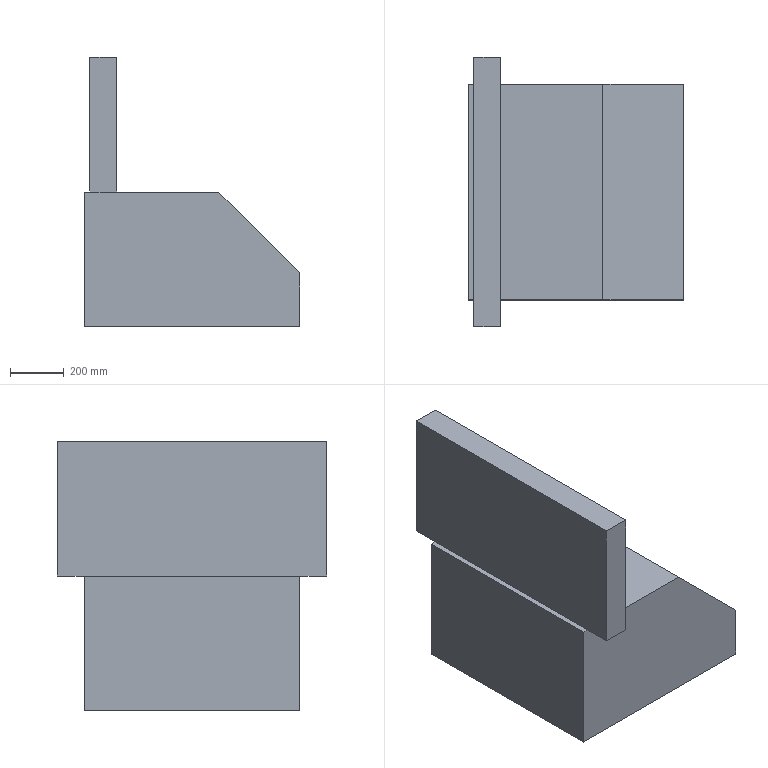Part | NX | features BREP 1 | 1 solid | 15 faces | box 800 x 1000 x 1000 mm | volume 334000000 mm3 | plane 15
STEP:
#1=CARTESIAN_POINT('',(400.,400.,0.));
#2=VERTEX_POINT('',#1);
#3=CARTESIAN_POINT('',(-400.,400.,0.));
#4=VERTEX_POINT('',#3);
#5=CARTESIAN_POINT('',(0.,400.,0.));
#6=DIRECTION('',(-1.,0.,0.));
#7=VECTOR('',#6,1000.);
#8=LINE('',#5,#7);
#9=EDGE_CURVE('',#2,#4,#8,.T.);
#10=ORIENTED_EDGE('',*,*,#9,.F.);
#11=CARTESIAN_POINT('',(400.,-400.,0.));
#12=VERTEX_POINT('',#11);
#13=CARTESIAN_POINT('',(400.,0.,0.));
#14=DIRECTION('',(0.,1.,0.));
#15=VECTOR('',#14,1000.);
#16=LINE('',#13,#15);
#17=EDGE_CURVE('',#12,#2,#16,.T.);
#18=ORIENTED_EDGE('',*,*,#17,.F.);
#19=CARTESIAN_POINT('',(-400.,-400.,0.));
#20=VERTEX_POINT('',#19);
#21=CARTESIAN_POINT('',(0.,-400.,0.));
#22=DIRECTION('',(1.,0.,0.));
#23=VECTOR('',#22,1000.);
#24=LINE('',#21,#23);
#25=EDGE_CURVE('',#20,#12,#24,.T.);
#26=ORIENTED_EDGE('',*,*,#25,.F.);
#27=CARTESIAN_POINT('',(-400.,0.,0.));
#28=DIRECTION('',(0.,-1.,0.));
#29=VECTOR('',#28,1000.);
#30=LINE('',#27,#29);
#31=EDGE_CURVE('',#4,#20,#30,.T.);
#32=ORIENTED_EDGE('',*,*,#31,.F.);
#33=EDGE_LOOP('',(#10,#18,#26,#32));
#34=FACE_BOUND('',#33,.T.);
#35=CARTESIAN_POINT('',(0.,0.,0.));
#36=DIRECTION('',(0.,0.,1.));
#37=DIRECTION('',(1.,0.,0.));
#38=AXIS2_PLACEMENT_3D('',#35,#36,#37);
#39=PLANE('',#38);
#40=ADVANCED_FACE('',(#34),#39,.F.);
#41=CARTESIAN_POINT('',(-400.,-400.,500.));
#42=VERTEX_POINT('',#41);
#43=CARTESIAN_POINT('',(-400.,-400.,500.));
#44=DIRECTION('',(0.,0.,-1.));
#45=VECTOR('',#44,1000.);
#46=LINE('',#43,#45);
#47=EDGE_CURVE('',#42,#20,#46,.T.);
#48=ORIENTED_EDGE('',*,*,#47,.F.);
#49=CARTESIAN_POINT('',(-400.,400.,500.));
#50=VERTEX_POINT('',#49);
#51=CARTESIAN_POINT('',(-400.,-400.,500.));
#52=DIRECTION('',(0.,-1.,0.));
#53=VECTOR('',#52,1000.);
#54=LINE('',#51,#53);
#55=EDGE_CURVE('',#50,#42,#54,.T.);
#56=ORIENTED_EDGE('',*,*,#55,.F.);
#57=CARTESIAN_POINT('',(-400.,400.,500.));
#58=DIRECTION('',(0.,0.,1.));
#59=VECTOR('',#58,1000.);
#60=LINE('',#57,#59);
#61=EDGE_CURVE('',#4,#50,#60,.T.);
#62=ORIENTED_EDGE('',*,*,#61,.F.);
#63=ORIENTED_EDGE('',*,*,#31,.T.);
#64=EDGE_LOOP('',(#48,#56,#62,#63));
#65=FACE_BOUND('',#64,.T.);
#66=CARTESIAN_POINT('',(-400.,-400.,500.));
#67=DIRECTION('',(1.,0.,0.));
#68=DIRECTION('',(0.,1.,0.));
#69=AXIS2_PLACEMENT_3D('',#66,#67,#68);
#70=PLANE('',#69);
#71=ADVANCED_FACE('',(#65),#70,.F.);
#72=CARTESIAN_POINT('',(400.,400.,200.));
#73=VERTEX_POINT('',#72);
#74=CARTESIAN_POINT('',(100.,400.,500.));
#75=VERTEX_POINT('',#74);
#76=CARTESIAN_POINT('',(400.,400.,200.));
#77=DIRECTION('',(-0.7071,0.,0.7071));
#78=VECTOR('',#77,1000.);
#79=LINE('',#76,#78);
#80=EDGE_CURVE('',#73,#75,#79,.T.);
#81=ORIENTED_EDGE('',*,*,#80,.F.);
#82=CARTESIAN_POINT('',(400.,400.,500.));
#83=DIRECTION('',(0.,0.,1.));
#84=VECTOR('',#83,1000.);
#85=LINE('',#82,#84);
#86=EDGE_CURVE('',#2,#73,#85,.T.);
#87=ORIENTED_EDGE('',*,*,#86,.F.);
#88=ORIENTED_EDGE('',*,*,#9,.T.);
#89=ORIENTED_EDGE('',*,*,#61,.T.);
#90=CARTESIAN_POINT('',(-380.,400.,500.));
#91=VERTEX_POINT('',#90);
#92=CARTESIAN_POINT('',(400.,400.,500.));
#93=DIRECTION('',(-1.,0.,0.));
#94=VECTOR('',#93,1000.);
#95=LINE('',#92,#94);
#96=EDGE_CURVE('',#91,#50,#95,.T.);
#97=ORIENTED_EDGE('',*,*,#96,.F.);
#98=CARTESIAN_POINT('',(-280.,400.,500.));
#99=VERTEX_POINT('',#98);
#100=CARTESIAN_POINT('',(400.,400.,500.));
#101=DIRECTION('',(-1.,0.,0.));
#102=VECTOR('',#101,1000.);
#103=LINE('',#100,#102);
#104=EDGE_CURVE('',#99,#91,#103,.T.);
#105=ORIENTED_EDGE('',*,*,#104,.F.);
#106=CARTESIAN_POINT('',(400.,400.,500.));
#107=DIRECTION('',(-1.,0.,0.));
#108=VECTOR('',#107,1000.);
#109=LINE('',#106,#108);
#110=EDGE_CURVE('',#75,#99,#109,.T.);
#111=ORIENTED_EDGE('',*,*,#110,.F.);
#112=EDGE_LOOP('',(#81,#87,#88,#89,#97,#105,#111));
#113=FACE_BOUND('',#112,.T.);
#114=CARTESIAN_POINT('',(400.,400.,500.));
#115=DIRECTION('',(0.,-1.,0.));
#116=DIRECTION('',(0.,0.,-1.));
#117=AXIS2_PLACEMENT_3D('',#114,#115,#116);
#118=PLANE('',#117);
#119=ADVANCED_FACE('',(#113),#118,.F.);
#120=CARTESIAN_POINT('',(400.,-400.,200.));
#121=VERTEX_POINT('',#120);
#122=CARTESIAN_POINT('',(400.,-400.,200.));
#123=DIRECTION('',(0.,1.,0.));
#124=VECTOR('',#123,1000.);
#125=LINE('',#122,#124);
#126=EDGE_CURVE('',#121,#73,#125,.T.);
#127=ORIENTED_EDGE('',*,*,#126,.F.);
#128=CARTESIAN_POINT('',(400.,-400.,500.));
#129=DIRECTION('',(0.,0.,1.));
#130=VECTOR('',#129,1000.);
#131=LINE('',#128,#130);
#132=EDGE_CURVE('',#12,#121,#131,.T.);
#133=ORIENTED_EDGE('',*,*,#132,.F.);
#134=ORIENTED_EDGE('',*,*,#17,.T.);
#135=ORIENTED_EDGE('',*,*,#86,.T.);
#136=EDGE_LOOP('',(#127,#133,#134,#135));
#137=FACE_BOUND('',#136,.T.);
#138=CARTESIAN_POINT('',(400.,-400.,500.));
#139=DIRECTION('',(-1.,0.,0.));
#140=DIRECTION('',(0.,0.,1.));
#141=AXIS2_PLACEMENT_3D('',#138,#139,#140);
#142=PLANE('',#141);
#143=ADVANCED_FACE('',(#137),#142,.F.);
#144=CARTESIAN_POINT('',(100.,-400.,500.));
#145=VERTEX_POINT('',#144);
#146=CARTESIAN_POINT('',(100.,-400.,500.));
#147=DIRECTION('',(0.7071,0.,-0.7071));
#148=VECTOR('',#147,1000.);
#149=LINE('',#146,#148);
#150=EDGE_CURVE('',#145,#121,#149,.T.);
#151=ORIENTED_EDGE('',*,*,#150,.F.);
#152=CARTESIAN_POINT('',(-280.,-400.,500.));
#153=VERTEX_POINT('',#152);
#154=CARTESIAN_POINT('',(400.,-400.,500.));
#155=DIRECTION('',(1.,0.,0.));
#156=VECTOR('',#155,1000.);
#157=LINE('',#154,#156);
#158=EDGE_CURVE('',#153,#145,#157,.T.);
#159=ORIENTED_EDGE('',*,*,#158,.F.);
#160=CARTESIAN_POINT('',(-380.,-400.,500.));
#161=VERTEX_POINT('',#160);
#162=CARTESIAN_POINT('',(400.,-400.,500.));
#163=DIRECTION('',(1.,0.,0.));
#164=VECTOR('',#163,1000.);
#165=LINE('',#162,#164);
#166=EDGE_CURVE('',#161,#153,#165,.T.);
#167=ORIENTED_EDGE('',*,*,#166,.F.);
#168=CARTESIAN_POINT('',(400.,-400.,500.));
#169=DIRECTION('',(1.,0.,0.));
#170=VECTOR('',#169,1000.);
#171=LINE('',#168,#170);
#172=EDGE_CURVE('',#42,#161,#171,.T.);
#173=ORIENTED_EDGE('',*,*,#172,.F.);
#174=ORIENTED_EDGE('',*,*,#47,.T.);
#175=ORIENTED_EDGE('',*,*,#25,.T.);
#176=ORIENTED_EDGE('',*,*,#132,.T.);
#177=EDGE_LOOP('',(#151,#159,#167,#173,#174,#175,#176));
#178=FACE_BOUND('',#177,.T.);
#179=CARTESIAN_POINT('',(400.,-400.,500.));
#180=DIRECTION('',(0.,1.,0.));
#181=DIRECTION('',(1.,0.,0.));
#182=AXIS2_PLACEMENT_3D('',#179,#180,#181);
#183=PLANE('',#182);
#184=ADVANCED_FACE('',(#178),#183,.F.);
#185=ORIENTED_EDGE('',*,*,#55,.T.);
#186=ORIENTED_EDGE('',*,*,#172,.T.);
#187=CARTESIAN_POINT('',(-380.,0.,500.));
#188=DIRECTION('',(0.,1.,0.));
#189=VECTOR('',#188,1000.);
#190=LINE('',#187,#189);
#191=EDGE_CURVE('',#161,#91,#190,.T.);
#192=ORIENTED_EDGE('',*,*,#191,.T.);
#193=ORIENTED_EDGE('',*,*,#96,.T.);
#194=EDGE_LOOP('',(#185,#186,#192,#193));
#195=FACE_BOUND('',#194,.T.);
#196=CARTESIAN_POINT('',(0.,0.,500.));
#197=DIRECTION('',(0.,0.,1.));
#198=DIRECTION('',(1.,0.,0.));
#199=AXIS2_PLACEMENT_3D('',#196,#197,#198);
#200=PLANE('',#199);
#201=ADVANCED_FACE('',(#195),#200,.T.);
#202=CARTESIAN_POINT('',(100.,0.,500.));
#203=DIRECTION('',(0.,1.,0.));
#204=VECTOR('',#203,1000.);
#205=LINE('',#202,#204);
#206=EDGE_CURVE('',#145,#75,#205,.T.);
#207=ORIENTED_EDGE('',*,*,#206,.T.);
#208=ORIENTED_EDGE('',*,*,#110,.T.);
#209=CARTESIAN_POINT('',(-280.,0.,500.));
#210=DIRECTION('',(0.,-1.,0.));
#211=VECTOR('',#210,1000.);
#212=LINE('',#209,#211);
#213=EDGE_CURVE('',#99,#153,#212,.T.);
#214=ORIENTED_EDGE('',*,*,#213,.T.);
#215=ORIENTED_EDGE('',*,*,#158,.T.);
#216=EDGE_LOOP('',(#207,#208,#214,#215));
#217=FACE_BOUND('',#216,.T.);
#218=CARTESIAN_POINT('',(0.,0.,500.));
#219=DIRECTION('',(0.,0.,1.));
#220=DIRECTION('',(1.,0.,0.));
#221=AXIS2_PLACEMENT_3D('',#218,#219,#220);
#222=PLANE('',#221);
#223=ADVANCED_FACE('',(#217),#222,.T.);
#224=ORIENTED_EDGE('',*,*,#80,.T.);
#225=ORIENTED_EDGE('',*,*,#206,.F.);
#226=ORIENTED_EDGE('',*,*,#150,.T.);
#227=ORIENTED_EDGE('',*,*,#126,.T.);
#228=EDGE_LOOP('',(#224,#225,#226,#227));
#229=FACE_BOUND('',#228,.T.);
#230=CARTESIAN_POINT('',(100.,0.,500.));
#231=DIRECTION('',(0.7071,0.,0.7071));
#232=DIRECTION('',(0.,-1.,0.));
#233=AXIS2_PLACEMENT_3D('',#230,#231,#232);
#234=PLANE('',#233);
#235=ADVANCED_FACE('',(#229),#234,.T.);
#236=ORIENTED_EDGE('',*,*,#104,.T.);
#237=CARTESIAN_POINT('',(-380.,500.,500.));
#238=VERTEX_POINT('',#237);
#239=CARTESIAN_POINT('',(-380.,0.,500.));
#240=DIRECTION('',(0.,-1.,0.));
#241=VECTOR('',#240,1000.);
#242=LINE('',#239,#241);
#243=EDGE_CURVE('',#238,#91,#242,.T.);
#244=ORIENTED_EDGE('',*,*,#243,.F.);
#245=CARTESIAN_POINT('',(-280.,500.,500.));
#246=VERTEX_POINT('',#245);
#247=CARTESIAN_POINT('',(0.,500.,500.));
#248=DIRECTION('',(-1.,0.,0.));
#249=VECTOR('',#248,1000.);
#250=LINE('',#247,#249);
#251=EDGE_CURVE('',#246,#238,#250,.T.);
#252=ORIENTED_EDGE('',*,*,#251,.F.);
#253=CARTESIAN_POINT('',(-280.,0.,500.));
#254=DIRECTION('',(0.,1.,0.));
#255=VECTOR('',#254,1000.);
#256=LINE('',#253,#255);
#257=EDGE_CURVE('',#99,#246,#256,.T.);
#258=ORIENTED_EDGE('',*,*,#257,.F.);
#259=EDGE_LOOP('',(#236,#244,#252,#258));
#260=FACE_BOUND('',#259,.T.);
#261=CARTESIAN_POINT('',(0.,0.,500.));
#262=DIRECTION('',(0.,0.,1.));
#263=DIRECTION('',(1.,0.,0.));
#264=AXIS2_PLACEMENT_3D('',#261,#262,#263);
#265=PLANE('',#264);
#266=ADVANCED_FACE('',(#260),#265,.F.);
#267=ORIENTED_EDGE('',*,*,#166,.T.);
#268=CARTESIAN_POINT('',(-280.,-500.,500.));
#269=VERTEX_POINT('',#268);
#270=CARTESIAN_POINT('',(-280.,0.,500.));
#271=DIRECTION('',(0.,1.,0.));
#272=VECTOR('',#271,1000.);
#273=LINE('',#270,#272);
#274=EDGE_CURVE('',#269,#153,#273,.T.);
#275=ORIENTED_EDGE('',*,*,#274,.F.);
#276=CARTESIAN_POINT('',(-380.,-500.,500.));
#277=VERTEX_POINT('',#276);
#278=CARTESIAN_POINT('',(0.,-500.,500.));
#279=DIRECTION('',(1.,0.,0.));
#280=VECTOR('',#279,1000.);
#281=LINE('',#278,#280);
#282=EDGE_CURVE('',#277,#269,#281,.T.);
#283=ORIENTED_EDGE('',*,*,#282,.F.);
#284=CARTESIAN_POINT('',(-380.,0.,500.));
#285=DIRECTION('',(0.,-1.,0.));
#286=VECTOR('',#285,1000.);
#287=LINE('',#284,#286);
#288=EDGE_CURVE('',#161,#277,#287,.T.);
#289=ORIENTED_EDGE('',*,*,#288,.F.);
#290=EDGE_LOOP('',(#267,#275,#283,#289));
#291=FACE_BOUND('',#290,.T.);
#292=CARTESIAN_POINT('',(0.,0.,500.));
#293=DIRECTION('',(0.,0.,1.));
#294=DIRECTION('',(1.,0.,0.));
#295=AXIS2_PLACEMENT_3D('',#292,#293,#294);
#296=PLANE('',#295);
#297=ADVANCED_FACE('',(#291),#296,.F.);
#298=ORIENTED_EDGE('',*,*,#191,.F.);
#299=ORIENTED_EDGE('',*,*,#288,.T.);
#300=CARTESIAN_POINT('',(-380.,-500.,1000.));
#301=VERTEX_POINT('',#300);
#302=CARTESIAN_POINT('',(-380.,-500.,1000.));
#303=DIRECTION('',(0.,0.,-1.));
#304=VECTOR('',#303,1000.);
#305=LINE('',#302,#304);
#306=EDGE_CURVE('',#301,#277,#305,.T.);
#307=ORIENTED_EDGE('',*,*,#306,.F.);
#308=CARTESIAN_POINT('',(-380.,500.,1000.));
#309=VERTEX_POINT('',#308);
#310=CARTESIAN_POINT('',(-380.,-500.,1000.));
#311=DIRECTION('',(0.,-1.,0.));
#312=VECTOR('',#311,1000.);
#313=LINE('',#310,#312);
#314=EDGE_CURVE('',#309,#301,#313,.T.);
#315=ORIENTED_EDGE('',*,*,#314,.F.);
#316=CARTESIAN_POINT('',(-380.,500.,1000.));
#317=DIRECTION('',(0.,0.,1.));
#318=VECTOR('',#317,1000.);
#319=LINE('',#316,#318);
#320=EDGE_CURVE('',#238,#309,#319,.T.);
#321=ORIENTED_EDGE('',*,*,#320,.F.);
#322=ORIENTED_EDGE('',*,*,#243,.T.);
#323=EDGE_LOOP('',(#298,#299,#307,#315,#321,#322));
#324=FACE_BOUND('',#323,.T.);
#325=CARTESIAN_POINT('',(-380.,-500.,1000.));
#326=DIRECTION('',(1.,0.,0.));
#327=DIRECTION('',(0.,1.,0.));
#328=AXIS2_PLACEMENT_3D('',#325,#326,#327);
#329=PLANE('',#328);
#330=ADVANCED_FACE('',(#324),#329,.F.);
#331=ORIENTED_EDGE('',*,*,#213,.F.);
#332=ORIENTED_EDGE('',*,*,#257,.T.);
#333=CARTESIAN_POINT('',(-280.,500.,1000.));
#334=VERTEX_POINT('',#333);
#335=CARTESIAN_POINT('',(-280.,500.,1000.));
#336=DIRECTION('',(0.,0.,-1.));
#337=VECTOR('',#336,1000.);
#338=LINE('',#335,#337);
#339=EDGE_CURVE('',#334,#246,#338,.T.);
#340=ORIENTED_EDGE('',*,*,#339,.F.);
#341=CARTESIAN_POINT('',(-280.,-500.,1000.));
#342=VERTEX_POINT('',#341);
#343=CARTESIAN_POINT('',(-280.,-500.,1000.));
#344=DIRECTION('',(0.,1.,0.));
#345=VECTOR('',#344,1000.);
#346=LINE('',#343,#345);
#347=EDGE_CURVE('',#342,#334,#346,.T.);
#348=ORIENTED_EDGE('',*,*,#347,.F.);
#349=CARTESIAN_POINT('',(-280.,-500.,1000.));
#350=DIRECTION('',(0.,0.,1.));
#351=VECTOR('',#350,1000.);
#352=LINE('',#349,#351);
#353=EDGE_CURVE('',#269,#342,#352,.T.);
#354=ORIENTED_EDGE('',*,*,#353,.F.);
#355=ORIENTED_EDGE('',*,*,#274,.T.);
#356=EDGE_LOOP('',(#331,#332,#340,#348,#354,#355));
#357=FACE_BOUND('',#356,.T.);
#358=CARTESIAN_POINT('',(-280.,-500.,1000.));
#359=DIRECTION('',(-1.,0.,0.));
#360=DIRECTION('',(0.,0.,1.));
#361=AXIS2_PLACEMENT_3D('',#358,#359,#360);
#362=PLANE('',#361);
#363=ADVANCED_FACE('',(#357),#362,.F.);
#364=ORIENTED_EDGE('',*,*,#320,.T.);
#365=CARTESIAN_POINT('',(-280.,500.,1000.));
#366=DIRECTION('',(-1.,0.,0.));
#367=VECTOR('',#366,1000.);
#368=LINE('',#365,#367);
#369=EDGE_CURVE('',#334,#309,#368,.T.);
#370=ORIENTED_EDGE('',*,*,#369,.F.);
#371=ORIENTED_EDGE('',*,*,#339,.T.);
#372=ORIENTED_EDGE('',*,*,#251,.T.);
#373=EDGE_LOOP('',(#364,#370,#371,#372));
#374=FACE_BOUND('',#373,.T.);
#375=CARTESIAN_POINT('',(-280.,500.,1000.));
#376=DIRECTION('',(0.,-1.,0.));
#377=DIRECTION('',(0.,0.,-1.));
#378=AXIS2_PLACEMENT_3D('',#375,#376,#377);
#379=PLANE('',#378);
#380=ADVANCED_FACE('',(#374),#379,.F.);
#381=ORIENTED_EDGE('',*,*,#353,.T.);
#382=CARTESIAN_POINT('',(-280.,-500.,1000.));
#383=DIRECTION('',(1.,0.,0.));
#384=VECTOR('',#383,1000.);
#385=LINE('',#382,#384);
#386=EDGE_CURVE('',#301,#342,#385,.T.);
#387=ORIENTED_EDGE('',*,*,#386,.F.);
#388=ORIENTED_EDGE('',*,*,#306,.T.);
#389=ORIENTED_EDGE('',*,*,#282,.T.);
#390=EDGE_LOOP('',(#381,#387,#388,#389));
#391=FACE_BOUND('',#390,.T.);
#392=CARTESIAN_POINT('',(-280.,-500.,1000.));
#393=DIRECTION('',(0.,1.,0.));
#394=DIRECTION('',(1.,0.,0.));
#395=AXIS2_PLACEMENT_3D('',#392,#393,#394);
#396=PLANE('',#395);
#397=ADVANCED_FACE('',(#391),#396,.F.);
#398=ORIENTED_EDGE('',*,*,#347,.T.);
#399=ORIENTED_EDGE('',*,*,#369,.T.);
#400=ORIENTED_EDGE('',*,*,#314,.T.);
#401=ORIENTED_EDGE('',*,*,#386,.T.);
#402=EDGE_LOOP('',(#398,#399,#400,#401));
#403=FACE_BOUND('',#402,.T.);
#404=CARTESIAN_POINT('',(0.,0.,1000.));
#405=DIRECTION('',(0.,0.,1.));
#406=DIRECTION('',(1.,0.,0.));
#407=AXIS2_PLACEMENT_3D('',#404,#405,#406);
#408=PLANE('',#407);
#409=ADVANCED_FACE('',(#403),#408,.T.);
#410=CLOSED_SHELL('',(#40,#71,#119,#143,#184,#201,#223,#235,#266,#297,#330,#363,#380,#397,#409));
#411=MANIFOLD_SOLID_BREP('',#410);
#412=(LENGTH_UNIT()NAMED_UNIT(*)SI_UNIT(.MILLI.,.METRE.));
#413=UNCERTAINTY_MEASURE_WITH_UNIT(LENGTH_MEASURE(0.00001),#412,'','');
#414=(NAMED_UNIT(*)PLANE_ANGLE_UNIT()SI_UNIT($,.RADIAN.));
#415=(NAMED_UNIT(*)SI_UNIT($,.STERADIAN.)SOLID_ANGLE_UNIT());
#416=(GEOMETRIC_REPRESENTATION_CONTEXT(3)GLOBAL_UNCERTAINTY_ASSIGNED_CONTEXT((#413))GLOBAL_UNIT_ASSIGNED_CONTEXT((#412,#414,#415))REPRESENTATION_CONTEXT('',''));
#417=ADVANCED_BREP_SHAPE_REPRESENTATION('',(#411),#416);